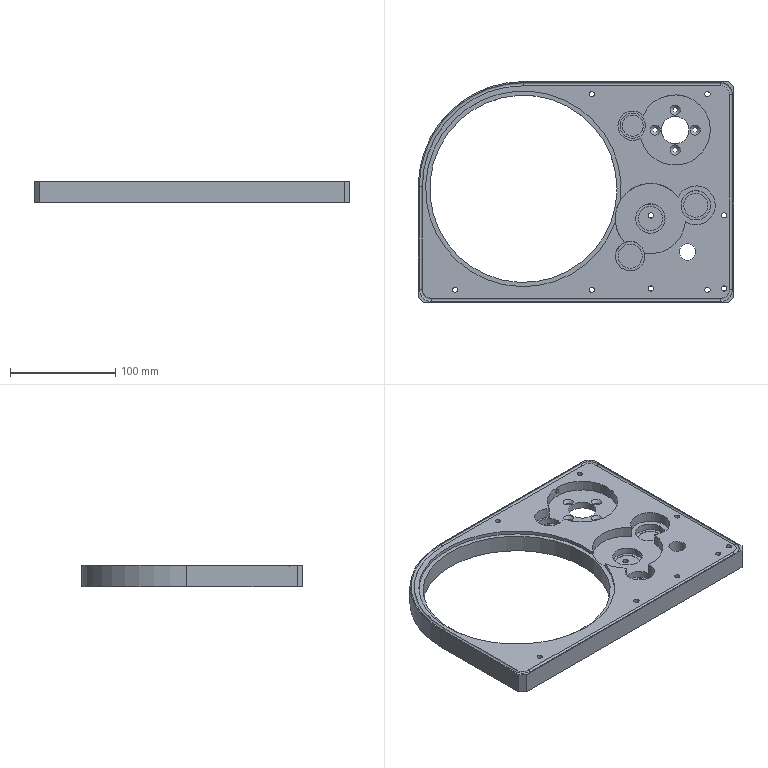Part | NX | features BREP 1 | 1 solid | 71 faces | box 300 x 210 x 20 mm | volume 576128 mm3 | cylinder 39 | plane 23 | cone 5 | torus 4 | commonest cylinder face diameters 5 x9 3 x4 4.3 x4 28 x4 23 x3 67 x3